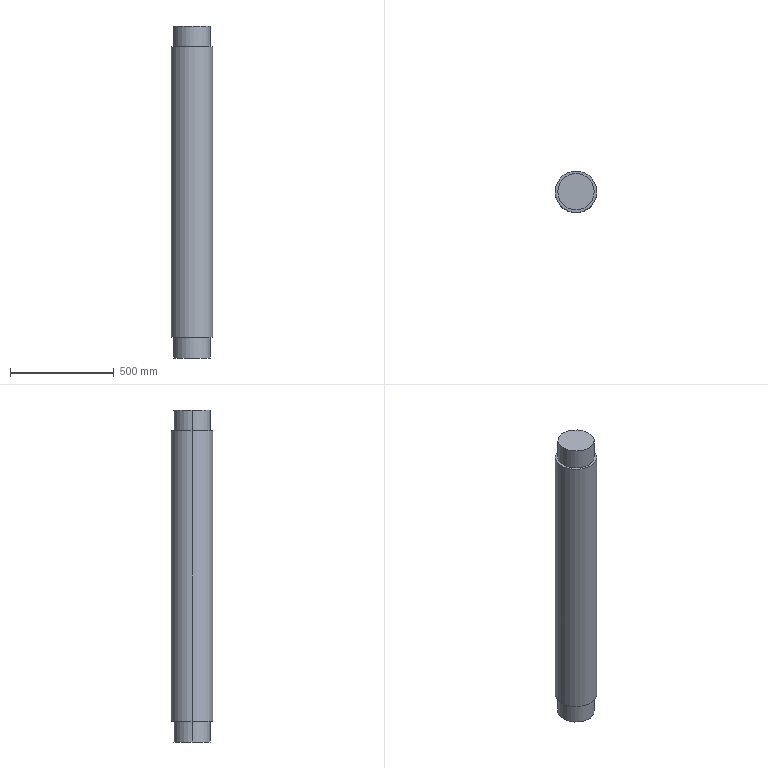Part | SolidWorks | features Extrusion 1, ICE 1 | 1 solid | 10 faces | box 200 x 200 x 1600 mm | volume 48792861 mm3 | cylinder 6 | plane 4 | commonest cylinder face diameters 175 x4 200 x2
STEP:
#1=CARTESIAN_POINT('',(87.5,0.,-700.));
#2=VERTEX_POINT('',#1);
#3=CARTESIAN_POINT('',(-87.5,0.,-700.));
#4=VERTEX_POINT('',#3);
#5=CARTESIAN_POINT('',(0.,0.,-700.));
#6=DIRECTION('',(0.,0.,1.));
#7=DIRECTION('',(1.,0.,0.));
#8=AXIS2_PLACEMENT_3D('',#5,#6,#7);
#9=CIRCLE('',#8,87.5);
#10=EDGE_CURVE('',#2,#4,#9,.T.);
#11=ORIENTED_EDGE('',*,*,#10,.F.);
#12=CARTESIAN_POINT('',(87.5,0.,-800.));
#13=VERTEX_POINT('',#12);
#14=CARTESIAN_POINT('',(87.5,0.,800.));
#15=DIRECTION('',(0.,0.,-1.));
#16=VECTOR('',#15,1000.);
#17=LINE('',#14,#16);
#18=EDGE_CURVE('',#2,#13,#17,.T.);
#19=ORIENTED_EDGE('',*,*,#18,.T.);
#20=CARTESIAN_POINT('',(-87.5,0.,-800.));
#21=VERTEX_POINT('',#20);
#22=CARTESIAN_POINT('',(0.,0.,-800.));
#23=DIRECTION('',(0.,0.,1.));
#24=DIRECTION('',(1.,0.,0.));
#25=AXIS2_PLACEMENT_3D('',#22,#23,#24);
#26=CIRCLE('',#25,87.5);
#27=EDGE_CURVE('',#13,#21,#26,.T.);
#28=ORIENTED_EDGE('',*,*,#27,.T.);
#29=CARTESIAN_POINT('',(-87.5,0.,800.));
#30=DIRECTION('',(0.,0.,-1.));
#31=VECTOR('',#30,1000.);
#32=LINE('',#29,#31);
#33=EDGE_CURVE('',#4,#21,#32,.T.);
#34=ORIENTED_EDGE('',*,*,#33,.F.);
#35=EDGE_LOOP('',(#11,#19,#28,#34));
#36=FACE_OUTER_BOUND('',#35,.T.);
#37=CARTESIAN_POINT('',(0.,0.,800.));
#38=DIRECTION('',(0.,0.,-1.));
#39=DIRECTION('',(-1.,0.,0.));
#40=AXIS2_PLACEMENT_3D('',#37,#38,#39);
#41=CYLINDRICAL_SURFACE('',#40,87.5);
#42=ADVANCED_FACE('',(#36),#41,.T.);
#43=CARTESIAN_POINT('',(100.,0.,700.));
#44=VERTEX_POINT('',#43);
#45=CARTESIAN_POINT('',(-100.,0.,700.));
#46=VERTEX_POINT('',#45);
#47=CARTESIAN_POINT('',(0.,0.,700.));
#48=DIRECTION('',(0.,0.,1.));
#49=DIRECTION('',(1.,0.,0.));
#50=AXIS2_PLACEMENT_3D('',#47,#48,#49);
#51=CIRCLE('',#50,100.);
#52=EDGE_CURVE('',#44,#46,#51,.T.);
#53=ORIENTED_EDGE('',*,*,#52,.F.);
#54=CARTESIAN_POINT('',(100.,0.,-700.));
#55=VERTEX_POINT('',#54);
#56=CARTESIAN_POINT('',(100.,0.,700.));
#57=DIRECTION('',(0.,0.,-1.));
#58=VECTOR('',#57,1000.);
#59=LINE('',#56,#58);
#60=EDGE_CURVE('',#44,#55,#59,.T.);
#61=ORIENTED_EDGE('',*,*,#60,.T.);
#62=CARTESIAN_POINT('',(-100.,0.,-700.));
#63=VERTEX_POINT('',#62);
#64=CARTESIAN_POINT('',(0.,0.,-700.));
#65=DIRECTION('',(0.,0.,1.));
#66=DIRECTION('',(1.,0.,0.));
#67=AXIS2_PLACEMENT_3D('',#64,#65,#66);
#68=CIRCLE('',#67,100.);
#69=EDGE_CURVE('',#55,#63,#68,.T.);
#70=ORIENTED_EDGE('',*,*,#69,.T.);
#71=CARTESIAN_POINT('',(-100.,0.,700.));
#72=DIRECTION('',(0.,0.,-1.));
#73=VECTOR('',#72,1000.);
#74=LINE('',#71,#73);
#75=EDGE_CURVE('',#46,#63,#74,.T.);
#76=ORIENTED_EDGE('',*,*,#75,.F.);
#77=EDGE_LOOP('',(#53,#61,#70,#76));
#78=FACE_OUTER_BOUND('',#77,.T.);
#79=CARTESIAN_POINT('',(0.,0.,700.));
#80=DIRECTION('',(0.,0.,-1.));
#81=DIRECTION('',(-1.,0.,0.));
#82=AXIS2_PLACEMENT_3D('',#79,#80,#81);
#83=CYLINDRICAL_SURFACE('',#82,100.);
#84=ADVANCED_FACE('',(#78),#83,.T.);
#85=CARTESIAN_POINT('',(87.5,0.,800.));
#86=VERTEX_POINT('',#85);
#87=CARTESIAN_POINT('',(-87.5,0.,800.));
#88=VERTEX_POINT('',#87);
#89=CARTESIAN_POINT('',(0.,0.,800.));
#90=DIRECTION('',(0.,0.,1.));
#91=DIRECTION('',(1.,0.,0.));
#92=AXIS2_PLACEMENT_3D('',#89,#90,#91);
#93=CIRCLE('',#92,87.5);
#94=EDGE_CURVE('',#86,#88,#93,.T.);
#95=ORIENTED_EDGE('',*,*,#94,.F.);
#96=CARTESIAN_POINT('',(87.5,0.,700.));
#97=VERTEX_POINT('',#96);
#98=CARTESIAN_POINT('',(87.5,0.,800.));
#99=DIRECTION('',(0.,0.,-1.));
#100=VECTOR('',#99,1000.);
#101=LINE('',#98,#100);
#102=EDGE_CURVE('',#86,#97,#101,.T.);
#103=ORIENTED_EDGE('',*,*,#102,.T.);
#104=CARTESIAN_POINT('',(-87.5,0.,700.));
#105=VERTEX_POINT('',#104);
#106=CARTESIAN_POINT('',(0.,0.,700.));
#107=DIRECTION('',(0.,0.,1.));
#108=DIRECTION('',(1.,0.,0.));
#109=AXIS2_PLACEMENT_3D('',#106,#107,#108);
#110=CIRCLE('',#109,87.5);
#111=EDGE_CURVE('',#97,#105,#110,.T.);
#112=ORIENTED_EDGE('',*,*,#111,.T.);
#113=CARTESIAN_POINT('',(-87.5,0.,800.));
#114=DIRECTION('',(0.,0.,-1.));
#115=VECTOR('',#114,1000.);
#116=LINE('',#113,#115);
#117=EDGE_CURVE('',#88,#105,#116,.T.);
#118=ORIENTED_EDGE('',*,*,#117,.F.);
#119=EDGE_LOOP('',(#95,#103,#112,#118));
#120=FACE_OUTER_BOUND('',#119,.T.);
#121=CARTESIAN_POINT('',(0.,0.,800.));
#122=DIRECTION('',(0.,0.,-1.));
#123=DIRECTION('',(-1.,0.,0.));
#124=AXIS2_PLACEMENT_3D('',#121,#122,#123);
#125=CYLINDRICAL_SURFACE('',#124,87.5);
#126=ADVANCED_FACE('',(#120),#125,.T.);
#127=ORIENTED_EDGE('',*,*,#102,.F.);
#128=CARTESIAN_POINT('',(0.,0.,800.));
#129=DIRECTION('',(0.,0.,1.));
#130=DIRECTION('',(1.,0.,0.));
#131=AXIS2_PLACEMENT_3D('',#128,#129,#130);
#132=CIRCLE('',#131,87.5);
#133=EDGE_CURVE('',#88,#86,#132,.T.);
#134=ORIENTED_EDGE('',*,*,#133,.F.);
#135=ORIENTED_EDGE('',*,*,#117,.T.);
#136=CARTESIAN_POINT('',(0.,0.,700.));
#137=DIRECTION('',(0.,0.,1.));
#138=DIRECTION('',(1.,0.,0.));
#139=AXIS2_PLACEMENT_3D('',#136,#137,#138);
#140=CIRCLE('',#139,87.5);
#141=EDGE_CURVE('',#105,#97,#140,.T.);
#142=ORIENTED_EDGE('',*,*,#141,.T.);
#143=EDGE_LOOP('',(#127,#134,#135,#142));
#144=FACE_OUTER_BOUND('',#143,.T.);
#145=CARTESIAN_POINT('',(0.,0.,800.));
#146=DIRECTION('',(0.,0.,-1.));
#147=DIRECTION('',(-1.,0.,0.));
#148=AXIS2_PLACEMENT_3D('',#145,#146,#147);
#149=CYLINDRICAL_SURFACE('',#148,87.5);
#150=ADVANCED_FACE('',(#144),#149,.T.);
#151=ORIENTED_EDGE('',*,*,#133,.T.);
#152=ORIENTED_EDGE('',*,*,#94,.T.);
#153=EDGE_LOOP('',(#151,#152));
#154=FACE_OUTER_BOUND('',#153,.T.);
#155=CARTESIAN_POINT('',(0.,0.,800.));
#156=DIRECTION('',(0.,0.,1.));
#157=DIRECTION('',(1.,0.,0.));
#158=AXIS2_PLACEMENT_3D('',#155,#156,#157);
#159=PLANE('',#158);
#160=ADVANCED_FACE('',(#154),#159,.T.);
#161=ORIENTED_EDGE('',*,*,#60,.F.);
#162=CARTESIAN_POINT('',(0.,0.,700.));
#163=DIRECTION('',(0.,0.,1.));
#164=DIRECTION('',(1.,0.,0.));
#165=AXIS2_PLACEMENT_3D('',#162,#163,#164);
#166=CIRCLE('',#165,100.);
#167=EDGE_CURVE('',#46,#44,#166,.T.);
#168=ORIENTED_EDGE('',*,*,#167,.F.);
#169=ORIENTED_EDGE('',*,*,#75,.T.);
#170=CARTESIAN_POINT('',(0.,0.,-700.));
#171=DIRECTION('',(0.,0.,1.));
#172=DIRECTION('',(1.,0.,0.));
#173=AXIS2_PLACEMENT_3D('',#170,#171,#172);
#174=CIRCLE('',#173,100.);
#175=EDGE_CURVE('',#63,#55,#174,.T.);
#176=ORIENTED_EDGE('',*,*,#175,.T.);
#177=EDGE_LOOP('',(#161,#168,#169,#176));
#178=FACE_OUTER_BOUND('',#177,.T.);
#179=CARTESIAN_POINT('',(0.,0.,700.));
#180=DIRECTION('',(0.,0.,-1.));
#181=DIRECTION('',(-1.,0.,0.));
#182=AXIS2_PLACEMENT_3D('',#179,#180,#181);
#183=CYLINDRICAL_SURFACE('',#182,100.);
#184=ADVANCED_FACE('',(#178),#183,.T.);
#185=ORIENTED_EDGE('',*,*,#141,.F.);
#186=ORIENTED_EDGE('',*,*,#111,.F.);
#187=EDGE_LOOP('',(#185,#186));
#188=FACE_BOUND('',#187,.T.);
#189=ORIENTED_EDGE('',*,*,#167,.T.);
#190=ORIENTED_EDGE('',*,*,#52,.T.);
#191=EDGE_LOOP('',(#189,#190));
#192=FACE_OUTER_BOUND('',#191,.T.);
#193=CARTESIAN_POINT('',(0.,0.,700.));
#194=DIRECTION('',(0.,0.,1.));
#195=DIRECTION('',(1.,0.,0.));
#196=AXIS2_PLACEMENT_3D('',#193,#194,#195);
#197=PLANE('',#196);
#198=ADVANCED_FACE('',(#188,#192),#197,.T.);
#199=CARTESIAN_POINT('',(0.,0.,-700.));
#200=DIRECTION('',(0.,0.,1.));
#201=DIRECTION('',(1.,0.,0.));
#202=AXIS2_PLACEMENT_3D('',#199,#200,#201);
#203=CIRCLE('',#202,87.5);
#204=EDGE_CURVE('',#4,#2,#203,.T.);
#205=ORIENTED_EDGE('',*,*,#204,.T.);
#206=ORIENTED_EDGE('',*,*,#10,.T.);
#207=EDGE_LOOP('',(#205,#206));
#208=FACE_BOUND('',#207,.T.);
#209=ORIENTED_EDGE('',*,*,#175,.F.);
#210=ORIENTED_EDGE('',*,*,#69,.F.);
#211=EDGE_LOOP('',(#209,#210));
#212=FACE_OUTER_BOUND('',#211,.T.);
#213=CARTESIAN_POINT('',(0.,0.,-700.));
#214=DIRECTION('',(0.,0.,1.));
#215=DIRECTION('',(1.,0.,0.));
#216=AXIS2_PLACEMENT_3D('',#213,#214,#215);
#217=PLANE('',#216);
#218=ADVANCED_FACE('',(#208,#212),#217,.F.);
#219=CARTESIAN_POINT('',(0.,0.,-800.));
#220=DIRECTION('',(0.,0.,1.));
#221=DIRECTION('',(1.,0.,0.));
#222=AXIS2_PLACEMENT_3D('',#219,#220,#221);
#223=CIRCLE('',#222,87.5);
#224=EDGE_CURVE('',#21,#13,#223,.T.);
#225=ORIENTED_EDGE('',*,*,#224,.F.);
#226=ORIENTED_EDGE('',*,*,#27,.F.);
#227=EDGE_LOOP('',(#225,#226));
#228=FACE_OUTER_BOUND('',#227,.T.);
#229=CARTESIAN_POINT('',(0.,0.,-800.));
#230=DIRECTION('',(0.,0.,1.));
#231=DIRECTION('',(1.,0.,0.));
#232=AXIS2_PLACEMENT_3D('',#229,#230,#231);
#233=PLANE('',#232);
#234=ADVANCED_FACE('',(#228),#233,.F.);
#235=ORIENTED_EDGE('',*,*,#18,.F.);
#236=ORIENTED_EDGE('',*,*,#204,.F.);
#237=ORIENTED_EDGE('',*,*,#33,.T.);
#238=ORIENTED_EDGE('',*,*,#224,.T.);
#239=EDGE_LOOP('',(#235,#236,#237,#238));
#240=FACE_OUTER_BOUND('',#239,.T.);
#241=CARTESIAN_POINT('',(0.,0.,800.));
#242=DIRECTION('',(0.,0.,-1.));
#243=DIRECTION('',(-1.,0.,0.));
#244=AXIS2_PLACEMENT_3D('',#241,#242,#243);
#245=CYLINDRICAL_SURFACE('',#244,87.5);
#246=ADVANCED_FACE('',(#240),#245,.T.);
#247=CLOSED_SHELL('',(#42,#84,#126,#150,#160,#184,#198,#218,#234,#246));
#248=MANIFOLD_SOLID_BREP('',#247);
#249=CARTESIAN_POINT('',(0.,0.,0.));
#250=DIRECTION('',(0.,0.,1.));
#251=DIRECTION('',(1.,0.,0.));
#252=AXIS2_PLACEMENT_3D('',#249,#250,#251);
#253=(LENGTH_UNIT()NAMED_UNIT(*)SI_UNIT(.MILLI.,.METRE.));
#254=UNCERTAINTY_MEASURE_WITH_UNIT(LENGTH_MEASURE(0.00001),#253,'','');
#255=(NAMED_UNIT(*)PLANE_ANGLE_UNIT()SI_UNIT($,.RADIAN.));
#256=(NAMED_UNIT(*)SI_UNIT($,.STERADIAN.)SOLID_ANGLE_UNIT());
#257=(GEOMETRIC_REPRESENTATION_CONTEXT(3)GLOBAL_UNCERTAINTY_ASSIGNED_CONTEXT((#254))GLOBAL_UNIT_ASSIGNED_CONTEXT((#253,#255,#256))REPRESENTATION_CONTEXT('',''));
#258=ADVANCED_BREP_SHAPE_REPRESENTATION('',(#248,#252),#257);